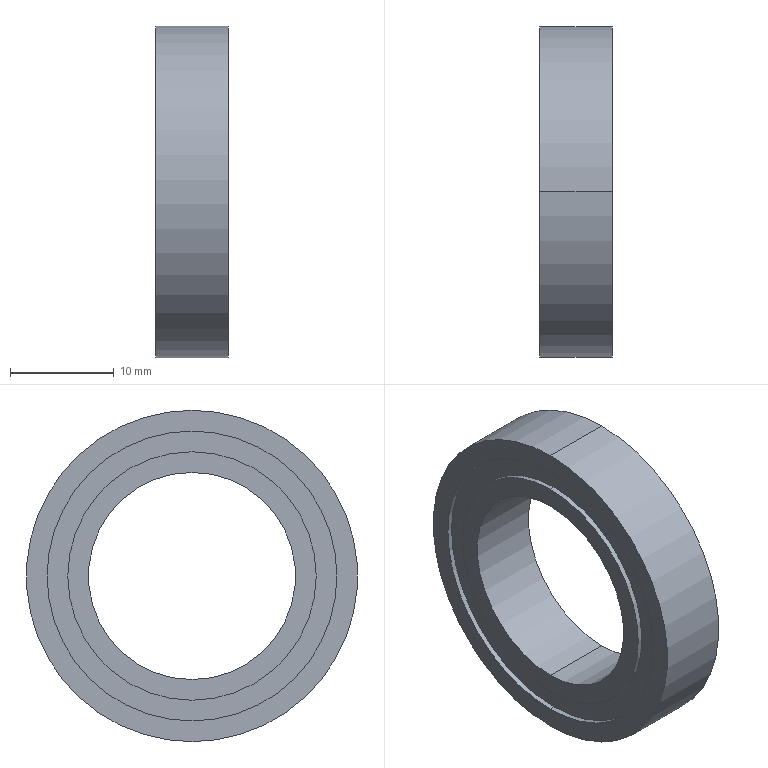Part | SolidWorks | features Revolution 1 | 1 solid | 18 faces | box 7 x 32 x 32 mm | volume 3267 mm3 | cylinder 12 | plane 6 | commonest cylinder face diameters 24 x4 28 x4 20 x2 32 x2
STEP:
#1=CARTESIAN_POINT('',(21.644,0.,-10.));
#2=VERTEX_POINT('',#1);
#3=CARTESIAN_POINT('',(21.644,0.,10.));
#4=VERTEX_POINT('',#3);
#5=CARTESIAN_POINT('',(21.644,0.,0.));
#6=DIRECTION('',(-1.,0.,0.));
#7=DIRECTION('',(0.,0.,1.));
#8=AXIS2_PLACEMENT_3D('',#5,#6,#7);
#9=CIRCLE('',#8,10.);
#10=EDGE_CURVE('',#2,#4,#9,.T.);
#11=ORIENTED_EDGE('',*,*,#10,.F.);
#12=CARTESIAN_POINT('',(14.644,0.,-10.));
#13=VERTEX_POINT('',#12);
#14=CARTESIAN_POINT('',(0.,0.,-10.));
#15=DIRECTION('',(-1.,0.,0.));
#16=VECTOR('',#15,1000.);
#17=LINE('',#14,#16);
#18=EDGE_CURVE('',#2,#13,#17,.T.);
#19=ORIENTED_EDGE('',*,*,#18,.T.);
#20=CARTESIAN_POINT('',(14.644,0.,10.));
#21=VERTEX_POINT('',#20);
#22=CARTESIAN_POINT('',(14.644,0.,0.));
#23=DIRECTION('',(-1.,0.,0.));
#24=DIRECTION('',(0.,0.,1.));
#25=AXIS2_PLACEMENT_3D('',#22,#23,#24);
#26=CIRCLE('',#25,10.);
#27=EDGE_CURVE('',#13,#21,#26,.T.);
#28=ORIENTED_EDGE('',*,*,#27,.T.);
#29=CARTESIAN_POINT('',(0.,0.,10.));
#30=DIRECTION('',(-1.,0.,0.));
#31=VECTOR('',#30,1000.);
#32=LINE('',#29,#31);
#33=EDGE_CURVE('',#4,#21,#32,.T.);
#34=ORIENTED_EDGE('',*,*,#33,.F.);
#35=EDGE_LOOP('',(#11,#19,#28,#34));
#36=FACE_OUTER_BOUND('',#35,.T.);
#37=CARTESIAN_POINT('',(0.,0.,0.));
#38=DIRECTION('',(-1.,0.,0.));
#39=DIRECTION('',(0.,0.,1.));
#40=AXIS2_PLACEMENT_3D('',#37,#38,#39);
#41=CYLINDRICAL_SURFACE('',#40,10.);
#42=ADVANCED_FACE('',(#36),#41,.F.);
#43=CARTESIAN_POINT('',(21.644,0.,12.));
#44=VERTEX_POINT('',#43);
#45=CARTESIAN_POINT('',(21.644,0.,-12.));
#46=VERTEX_POINT('',#45);
#47=CARTESIAN_POINT('',(21.644,0.,0.));
#48=DIRECTION('',(-1.,0.,0.));
#49=DIRECTION('',(0.,0.,1.));
#50=AXIS2_PLACEMENT_3D('',#47,#48,#49);
#51=CIRCLE('',#50,12.);
#52=EDGE_CURVE('',#44,#46,#51,.T.);
#53=ORIENTED_EDGE('',*,*,#52,.T.);
#54=CARTESIAN_POINT('',(21.144,0.,-12.));
#55=VERTEX_POINT('',#54);
#56=CARTESIAN_POINT('',(0.,0.,-12.));
#57=DIRECTION('',(-1.,0.,0.));
#58=VECTOR('',#57,1000.);
#59=LINE('',#56,#58);
#60=EDGE_CURVE('',#46,#55,#59,.T.);
#61=ORIENTED_EDGE('',*,*,#60,.T.);
#62=CARTESIAN_POINT('',(21.144,0.,12.));
#63=VERTEX_POINT('',#62);
#64=CARTESIAN_POINT('',(21.144,0.,0.));
#65=DIRECTION('',(-1.,0.,0.));
#66=DIRECTION('',(0.,0.,1.));
#67=AXIS2_PLACEMENT_3D('',#64,#65,#66);
#68=CIRCLE('',#67,12.);
#69=EDGE_CURVE('',#63,#55,#68,.T.);
#70=ORIENTED_EDGE('',*,*,#69,.F.);
#71=CARTESIAN_POINT('',(0.,0.,12.));
#72=DIRECTION('',(-1.,0.,0.));
#73=VECTOR('',#72,1000.);
#74=LINE('',#71,#73);
#75=EDGE_CURVE('',#44,#63,#74,.T.);
#76=ORIENTED_EDGE('',*,*,#75,.F.);
#77=EDGE_LOOP('',(#53,#61,#70,#76));
#78=FACE_OUTER_BOUND('',#77,.T.);
#79=CARTESIAN_POINT('',(0.,0.,0.));
#80=DIRECTION('',(-1.,0.,0.));
#81=DIRECTION('',(0.,0.,1.));
#82=AXIS2_PLACEMENT_3D('',#79,#80,#81);
#83=CYLINDRICAL_SURFACE('',#82,12.);
#84=ADVANCED_FACE('',(#78),#83,.T.);
#85=CARTESIAN_POINT('',(21.644,0.,-14.));
#86=VERTEX_POINT('',#85);
#87=CARTESIAN_POINT('',(21.644,0.,14.));
#88=VERTEX_POINT('',#87);
#89=CARTESIAN_POINT('',(21.644,0.,0.));
#90=DIRECTION('',(-1.,0.,0.));
#91=DIRECTION('',(0.,0.,1.));
#92=AXIS2_PLACEMENT_3D('',#89,#90,#91);
#93=CIRCLE('',#92,14.);
#94=EDGE_CURVE('',#86,#88,#93,.T.);
#95=ORIENTED_EDGE('',*,*,#94,.F.);
#96=CARTESIAN_POINT('',(21.144,0.,-14.));
#97=VERTEX_POINT('',#96);
#98=CARTESIAN_POINT('',(0.,0.,-14.));
#99=DIRECTION('',(-1.,0.,0.));
#100=VECTOR('',#99,1000.);
#101=LINE('',#98,#100);
#102=EDGE_CURVE('',#86,#97,#101,.T.);
#103=ORIENTED_EDGE('',*,*,#102,.T.);
#104=CARTESIAN_POINT('',(21.144,0.,14.));
#105=VERTEX_POINT('',#104);
#106=CARTESIAN_POINT('',(21.144,0.,0.));
#107=DIRECTION('',(-1.,0.,0.));
#108=DIRECTION('',(0.,0.,1.));
#109=AXIS2_PLACEMENT_3D('',#106,#107,#108);
#110=CIRCLE('',#109,14.);
#111=EDGE_CURVE('',#97,#105,#110,.T.);
#112=ORIENTED_EDGE('',*,*,#111,.T.);
#113=CARTESIAN_POINT('',(0.,0.,14.));
#114=DIRECTION('',(-1.,0.,0.));
#115=VECTOR('',#114,1000.);
#116=LINE('',#113,#115);
#117=EDGE_CURVE('',#88,#105,#116,.T.);
#118=ORIENTED_EDGE('',*,*,#117,.F.);
#119=EDGE_LOOP('',(#95,#103,#112,#118));
#120=FACE_OUTER_BOUND('',#119,.T.);
#121=CARTESIAN_POINT('',(0.,0.,0.));
#122=DIRECTION('',(-1.,0.,0.));
#123=DIRECTION('',(0.,0.,1.));
#124=AXIS2_PLACEMENT_3D('',#121,#122,#123);
#125=CYLINDRICAL_SURFACE('',#124,14.);
#126=ADVANCED_FACE('',(#120),#125,.F.);
#127=CARTESIAN_POINT('',(21.644,0.,16.));
#128=VERTEX_POINT('',#127);
#129=CARTESIAN_POINT('',(21.644,0.,-16.));
#130=VERTEX_POINT('',#129);
#131=CARTESIAN_POINT('',(21.644,0.,0.));
#132=DIRECTION('',(-1.,0.,0.));
#133=DIRECTION('',(0.,0.,1.));
#134=AXIS2_PLACEMENT_3D('',#131,#132,#133);
#135=CIRCLE('',#134,16.);
#136=EDGE_CURVE('',#128,#130,#135,.T.);
#137=ORIENTED_EDGE('',*,*,#136,.T.);
#138=CARTESIAN_POINT('',(14.644,0.,-16.));
#139=VERTEX_POINT('',#138);
#140=CARTESIAN_POINT('',(0.,0.,-16.));
#141=DIRECTION('',(-1.,0.,0.));
#142=VECTOR('',#141,1000.);
#143=LINE('',#140,#142);
#144=EDGE_CURVE('',#130,#139,#143,.T.);
#145=ORIENTED_EDGE('',*,*,#144,.T.);
#146=CARTESIAN_POINT('',(14.644,0.,16.));
#147=VERTEX_POINT('',#146);
#148=CARTESIAN_POINT('',(14.644,0.,0.));
#149=DIRECTION('',(-1.,0.,0.));
#150=DIRECTION('',(0.,0.,1.));
#151=AXIS2_PLACEMENT_3D('',#148,#149,#150);
#152=CIRCLE('',#151,16.);
#153=EDGE_CURVE('',#147,#139,#152,.T.);
#154=ORIENTED_EDGE('',*,*,#153,.F.);
#155=CARTESIAN_POINT('',(0.,0.,16.));
#156=DIRECTION('',(-1.,0.,0.));
#157=VECTOR('',#156,1000.);
#158=LINE('',#155,#157);
#159=EDGE_CURVE('',#128,#147,#158,.T.);
#160=ORIENTED_EDGE('',*,*,#159,.F.);
#161=EDGE_LOOP('',(#137,#145,#154,#160));
#162=FACE_OUTER_BOUND('',#161,.T.);
#163=CARTESIAN_POINT('',(0.,0.,0.));
#164=DIRECTION('',(-1.,0.,0.));
#165=DIRECTION('',(0.,0.,1.));
#166=AXIS2_PLACEMENT_3D('',#163,#164,#165);
#167=CYLINDRICAL_SURFACE('',#166,16.);
#168=ADVANCED_FACE('',(#162),#167,.T.);
#169=CARTESIAN_POINT('',(15.144,0.,-14.));
#170=VERTEX_POINT('',#169);
#171=CARTESIAN_POINT('',(15.144,0.,14.));
#172=VERTEX_POINT('',#171);
#173=CARTESIAN_POINT('',(15.144,0.,0.));
#174=DIRECTION('',(-1.,0.,0.));
#175=DIRECTION('',(0.,0.,1.));
#176=AXIS2_PLACEMENT_3D('',#173,#174,#175);
#177=CIRCLE('',#176,14.);
#178=EDGE_CURVE('',#170,#172,#177,.T.);
#179=ORIENTED_EDGE('',*,*,#178,.F.);
#180=CARTESIAN_POINT('',(14.644,0.,-14.));
#181=VERTEX_POINT('',#180);
#182=CARTESIAN_POINT('',(0.,0.,-14.));
#183=DIRECTION('',(-1.,0.,0.));
#184=VECTOR('',#183,1000.);
#185=LINE('',#182,#184);
#186=EDGE_CURVE('',#170,#181,#185,.T.);
#187=ORIENTED_EDGE('',*,*,#186,.T.);
#188=CARTESIAN_POINT('',(14.644,0.,14.));
#189=VERTEX_POINT('',#188);
#190=CARTESIAN_POINT('',(14.644,0.,0.));
#191=DIRECTION('',(-1.,0.,0.));
#192=DIRECTION('',(0.,0.,1.));
#193=AXIS2_PLACEMENT_3D('',#190,#191,#192);
#194=CIRCLE('',#193,14.);
#195=EDGE_CURVE('',#181,#189,#194,.T.);
#196=ORIENTED_EDGE('',*,*,#195,.T.);
#197=CARTESIAN_POINT('',(0.,0.,14.));
#198=DIRECTION('',(-1.,0.,0.));
#199=VECTOR('',#198,1000.);
#200=LINE('',#197,#199);
#201=EDGE_CURVE('',#172,#189,#200,.T.);
#202=ORIENTED_EDGE('',*,*,#201,.F.);
#203=EDGE_LOOP('',(#179,#187,#196,#202));
#204=FACE_OUTER_BOUND('',#203,.T.);
#205=CARTESIAN_POINT('',(0.,0.,0.));
#206=DIRECTION('',(-1.,0.,0.));
#207=DIRECTION('',(0.,0.,1.));
#208=AXIS2_PLACEMENT_3D('',#205,#206,#207);
#209=CYLINDRICAL_SURFACE('',#208,14.);
#210=ADVANCED_FACE('',(#204),#209,.F.);
#211=CARTESIAN_POINT('',(15.144,0.,12.));
#212=VERTEX_POINT('',#211);
#213=CARTESIAN_POINT('',(15.144,0.,-12.));
#214=VERTEX_POINT('',#213);
#215=CARTESIAN_POINT('',(15.144,0.,0.));
#216=DIRECTION('',(-1.,0.,0.));
#217=DIRECTION('',(0.,0.,1.));
#218=AXIS2_PLACEMENT_3D('',#215,#216,#217);
#219=CIRCLE('',#218,12.);
#220=EDGE_CURVE('',#212,#214,#219,.T.);
#221=ORIENTED_EDGE('',*,*,#220,.T.);
#222=CARTESIAN_POINT('',(14.644,0.,-12.));
#223=VERTEX_POINT('',#222);
#224=CARTESIAN_POINT('',(0.,0.,-12.));
#225=DIRECTION('',(-1.,0.,0.));
#226=VECTOR('',#225,1000.);
#227=LINE('',#224,#226);
#228=EDGE_CURVE('',#214,#223,#227,.T.);
#229=ORIENTED_EDGE('',*,*,#228,.T.);
#230=CARTESIAN_POINT('',(14.644,0.,12.));
#231=VERTEX_POINT('',#230);
#232=CARTESIAN_POINT('',(14.644,0.,0.));
#233=DIRECTION('',(-1.,0.,0.));
#234=DIRECTION('',(0.,0.,1.));
#235=AXIS2_PLACEMENT_3D('',#232,#233,#234);
#236=CIRCLE('',#235,12.);
#237=EDGE_CURVE('',#231,#223,#236,.T.);
#238=ORIENTED_EDGE('',*,*,#237,.F.);
#239=CARTESIAN_POINT('',(0.,0.,12.));
#240=DIRECTION('',(-1.,0.,0.));
#241=VECTOR('',#240,1000.);
#242=LINE('',#239,#241);
#243=EDGE_CURVE('',#212,#231,#242,.T.);
#244=ORIENTED_EDGE('',*,*,#243,.F.);
#245=EDGE_LOOP('',(#221,#229,#238,#244));
#246=FACE_OUTER_BOUND('',#245,.T.);
#247=CARTESIAN_POINT('',(0.,0.,0.));
#248=DIRECTION('',(-1.,0.,0.));
#249=DIRECTION('',(0.,0.,1.));
#250=AXIS2_PLACEMENT_3D('',#247,#248,#249);
#251=CYLINDRICAL_SURFACE('',#250,12.);
#252=ADVANCED_FACE('',(#246),#251,.T.);
#253=CARTESIAN_POINT('',(14.644,0.,0.));
#254=DIRECTION('',(-1.,0.,0.));
#255=DIRECTION('',(0.,0.,1.));
#256=AXIS2_PLACEMENT_3D('',#253,#254,#255);
#257=CIRCLE('',#256,10.);
#258=EDGE_CURVE('',#21,#13,#257,.T.);
#259=ORIENTED_EDGE('',*,*,#258,.F.);
#260=ORIENTED_EDGE('',*,*,#27,.F.);
#261=EDGE_LOOP('',(#259,#260));
#262=FACE_BOUND('',#261,.T.);
#263=ORIENTED_EDGE('',*,*,#237,.T.);
#264=CARTESIAN_POINT('',(14.644,0.,0.));
#265=DIRECTION('',(-1.,0.,0.));
#266=DIRECTION('',(0.,0.,1.));
#267=AXIS2_PLACEMENT_3D('',#264,#265,#266);
#268=CIRCLE('',#267,12.);
#269=EDGE_CURVE('',#223,#231,#268,.T.);
#270=ORIENTED_EDGE('',*,*,#269,.T.);
#271=EDGE_LOOP('',(#263,#270));
#272=FACE_OUTER_BOUND('',#271,.T.);
#273=CARTESIAN_POINT('',(14.644,10.,0.));
#274=DIRECTION('',(1.,0.,0.));
#275=DIRECTION('',(0.,0.,-1.));
#276=AXIS2_PLACEMENT_3D('',#273,#274,#275);
#277=PLANE('',#276);
#278=ADVANCED_FACE('',(#262,#272),#277,.F.);
#279=ORIENTED_EDGE('',*,*,#228,.F.);
#280=CARTESIAN_POINT('',(15.144,0.,0.));
#281=DIRECTION('',(-1.,0.,0.));
#282=DIRECTION('',(0.,0.,1.));
#283=AXIS2_PLACEMENT_3D('',#280,#281,#282);
#284=CIRCLE('',#283,12.);
#285=EDGE_CURVE('',#214,#212,#284,.T.);
#286=ORIENTED_EDGE('',*,*,#285,.T.);
#287=ORIENTED_EDGE('',*,*,#243,.T.);
#288=ORIENTED_EDGE('',*,*,#269,.F.);
#289=EDGE_LOOP('',(#279,#286,#287,#288));
#290=FACE_OUTER_BOUND('',#289,.T.);
#291=CARTESIAN_POINT('',(0.,0.,0.));
#292=DIRECTION('',(-1.,0.,0.));
#293=DIRECTION('',(0.,0.,1.));
#294=AXIS2_PLACEMENT_3D('',#291,#292,#293);
#295=CYLINDRICAL_SURFACE('',#294,12.);
#296=ADVANCED_FACE('',(#290),#295,.T.);
#297=ORIENTED_EDGE('',*,*,#220,.F.);
#298=ORIENTED_EDGE('',*,*,#285,.F.);
#299=EDGE_LOOP('',(#297,#298));
#300=FACE_BOUND('',#299,.T.);
#301=CARTESIAN_POINT('',(15.144,0.,0.));
#302=DIRECTION('',(-1.,0.,0.));
#303=DIRECTION('',(0.,0.,1.));
#304=AXIS2_PLACEMENT_3D('',#301,#302,#303);
#305=CIRCLE('',#304,14.);
#306=EDGE_CURVE('',#172,#170,#305,.T.);
#307=ORIENTED_EDGE('',*,*,#306,.T.);
#308=ORIENTED_EDGE('',*,*,#178,.T.);
#309=EDGE_LOOP('',(#307,#308));
#310=FACE_OUTER_BOUND('',#309,.T.);
#311=CARTESIAN_POINT('',(15.144,12.,0.));
#312=DIRECTION('',(1.,0.,0.));
#313=DIRECTION('',(0.,0.,-1.));
#314=AXIS2_PLACEMENT_3D('',#311,#312,#313);
#315=PLANE('',#314);
#316=ADVANCED_FACE('',(#300,#310),#315,.F.);
#317=ORIENTED_EDGE('',*,*,#186,.F.);
#318=ORIENTED_EDGE('',*,*,#306,.F.);
#319=ORIENTED_EDGE('',*,*,#201,.T.);
#320=CARTESIAN_POINT('',(14.644,0.,0.));
#321=DIRECTION('',(-1.,0.,0.));
#322=DIRECTION('',(0.,0.,1.));
#323=AXIS2_PLACEMENT_3D('',#320,#321,#322);
#324=CIRCLE('',#323,14.);
#325=EDGE_CURVE('',#189,#181,#324,.T.);
#326=ORIENTED_EDGE('',*,*,#325,.T.);
#327=EDGE_LOOP('',(#317,#318,#319,#326));
#328=FACE_OUTER_BOUND('',#327,.T.);
#329=CARTESIAN_POINT('',(0.,0.,0.));
#330=DIRECTION('',(-1.,0.,0.));
#331=DIRECTION('',(0.,0.,1.));
#332=AXIS2_PLACEMENT_3D('',#329,#330,#331);
#333=CYLINDRICAL_SURFACE('',#332,14.);
#334=ADVANCED_FACE('',(#328),#333,.F.);
#335=ORIENTED_EDGE('',*,*,#325,.F.);
#336=ORIENTED_EDGE('',*,*,#195,.F.);
#337=EDGE_LOOP('',(#335,#336));
#338=FACE_BOUND('',#337,.T.);
#339=ORIENTED_EDGE('',*,*,#153,.T.);
#340=CARTESIAN_POINT('',(14.644,0.,0.));
#341=DIRECTION('',(-1.,0.,0.));
#342=DIRECTION('',(0.,0.,1.));
#343=AXIS2_PLACEMENT_3D('',#340,#341,#342);
#344=CIRCLE('',#343,16.);
#345=EDGE_CURVE('',#139,#147,#344,.T.);
#346=ORIENTED_EDGE('',*,*,#345,.T.);
#347=EDGE_LOOP('',(#339,#346));
#348=FACE_OUTER_BOUND('',#347,.T.);
#349=CARTESIAN_POINT('',(14.644,14.,0.));
#350=DIRECTION('',(1.,0.,0.));
#351=DIRECTION('',(0.,0.,-1.));
#352=AXIS2_PLACEMENT_3D('',#349,#350,#351);
#353=PLANE('',#352);
#354=ADVANCED_FACE('',(#338,#348),#353,.F.);
#355=ORIENTED_EDGE('',*,*,#144,.F.);
#356=CARTESIAN_POINT('',(21.644,0.,0.));
#357=DIRECTION('',(-1.,0.,0.));
#358=DIRECTION('',(0.,0.,1.));
#359=AXIS2_PLACEMENT_3D('',#356,#357,#358);
#360=CIRCLE('',#359,16.);
#361=EDGE_CURVE('',#130,#128,#360,.T.);
#362=ORIENTED_EDGE('',*,*,#361,.T.);
#363=ORIENTED_EDGE('',*,*,#159,.T.);
#364=ORIENTED_EDGE('',*,*,#345,.F.);
#365=EDGE_LOOP('',(#355,#362,#363,#364));
#366=FACE_OUTER_BOUND('',#365,.T.);
#367=CARTESIAN_POINT('',(0.,0.,0.));
#368=DIRECTION('',(-1.,0.,0.));
#369=DIRECTION('',(0.,0.,1.));
#370=AXIS2_PLACEMENT_3D('',#367,#368,#369);
#371=CYLINDRICAL_SURFACE('',#370,16.);
#372=ADVANCED_FACE('',(#366),#371,.T.);
#373=ORIENTED_EDGE('',*,*,#136,.F.);
#374=ORIENTED_EDGE('',*,*,#361,.F.);
#375=EDGE_LOOP('',(#373,#374));
#376=FACE_OUTER_BOUND('',#375,.T.);
#377=CARTESIAN_POINT('',(21.644,0.,0.));
#378=DIRECTION('',(-1.,0.,0.));
#379=DIRECTION('',(0.,0.,1.));
#380=AXIS2_PLACEMENT_3D('',#377,#378,#379);
#381=CIRCLE('',#380,14.);
#382=EDGE_CURVE('',#88,#86,#381,.T.);
#383=ORIENTED_EDGE('',*,*,#382,.T.);
#384=ORIENTED_EDGE('',*,*,#94,.T.);
#385=EDGE_LOOP('',(#383,#384));
#386=FACE_BOUND('',#385,.T.);
#387=CARTESIAN_POINT('',(21.644,14.,0.));
#388=DIRECTION('',(-1.,0.,0.));
#389=DIRECTION('',(0.,0.,1.));
#390=AXIS2_PLACEMENT_3D('',#387,#388,#389);
#391=PLANE('',#390);
#392=ADVANCED_FACE('',(#376,#386),#391,.F.);
#393=ORIENTED_EDGE('',*,*,#102,.F.);
#394=ORIENTED_EDGE('',*,*,#382,.F.);
#395=ORIENTED_EDGE('',*,*,#117,.T.);
#396=CARTESIAN_POINT('',(21.144,0.,0.));
#397=DIRECTION('',(-1.,0.,0.));
#398=DIRECTION('',(0.,0.,1.));
#399=AXIS2_PLACEMENT_3D('',#396,#397,#398);
#400=CIRCLE('',#399,14.);
#401=EDGE_CURVE('',#105,#97,#400,.T.);
#402=ORIENTED_EDGE('',*,*,#401,.T.);
#403=EDGE_LOOP('',(#393,#394,#395,#402));
#404=FACE_OUTER_BOUND('',#403,.T.);
#405=CARTESIAN_POINT('',(0.,0.,0.));
#406=DIRECTION('',(-1.,0.,0.));
#407=DIRECTION('',(0.,0.,1.));
#408=AXIS2_PLACEMENT_3D('',#405,#406,#407);
#409=CYLINDRICAL_SURFACE('',#408,14.);
#410=ADVANCED_FACE('',(#404),#409,.F.);
#411=ORIENTED_EDGE('',*,*,#401,.F.);
#412=ORIENTED_EDGE('',*,*,#111,.F.);
#413=EDGE_LOOP('',(#411,#412));
#414=FACE_OUTER_BOUND('',#413,.T.);
#415=ORIENTED_EDGE('',*,*,#69,.T.);
#416=CARTESIAN_POINT('',(21.144,0.,0.));
#417=DIRECTION('',(-1.,0.,0.));
#418=DIRECTION('',(0.,0.,1.));
#419=AXIS2_PLACEMENT_3D('',#416,#417,#418);
#420=CIRCLE('',#419,12.);
#421=EDGE_CURVE('',#55,#63,#420,.T.);
#422=ORIENTED_EDGE('',*,*,#421,.T.);
#423=EDGE_LOOP('',(#415,#422));
#424=FACE_BOUND('',#423,.T.);
#425=CARTESIAN_POINT('',(21.144,12.,0.));
#426=DIRECTION('',(-1.,0.,0.));
#427=DIRECTION('',(0.,0.,1.));
#428=AXIS2_PLACEMENT_3D('',#425,#426,#427);
#429=PLANE('',#428);
#430=ADVANCED_FACE('',(#414,#424),#429,.F.);
#431=ORIENTED_EDGE('',*,*,#60,.F.);
#432=CARTESIAN_POINT('',(21.644,0.,0.));
#433=DIRECTION('',(-1.,0.,0.));
#434=DIRECTION('',(0.,0.,1.));
#435=AXIS2_PLACEMENT_3D('',#432,#433,#434);
#436=CIRCLE('',#435,12.);
#437=EDGE_CURVE('',#46,#44,#436,.T.);
#438=ORIENTED_EDGE('',*,*,#437,.T.);
#439=ORIENTED_EDGE('',*,*,#75,.T.);
#440=ORIENTED_EDGE('',*,*,#421,.F.);
#441=EDGE_LOOP('',(#431,#438,#439,#440));
#442=FACE_OUTER_BOUND('',#441,.T.);
#443=CARTESIAN_POINT('',(0.,0.,0.));
#444=DIRECTION('',(-1.,0.,0.));
#445=DIRECTION('',(0.,0.,1.));
#446=AXIS2_PLACEMENT_3D('',#443,#444,#445);
#447=CYLINDRICAL_SURFACE('',#446,12.);
#448=ADVANCED_FACE('',(#442),#447,.T.);
#449=ORIENTED_EDGE('',*,*,#52,.F.);
#450=ORIENTED_EDGE('',*,*,#437,.F.);
#451=EDGE_LOOP('',(#449,#450));
#452=FACE_OUTER_BOUND('',#451,.T.);
#453=CARTESIAN_POINT('',(21.644,0.,0.));
#454=DIRECTION('',(-1.,0.,0.));
#455=DIRECTION('',(0.,0.,1.));
#456=AXIS2_PLACEMENT_3D('',#453,#454,#455);
#457=CIRCLE('',#456,10.);
#458=EDGE_CURVE('',#4,#2,#457,.T.);
#459=ORIENTED_EDGE('',*,*,#458,.T.);
#460=ORIENTED_EDGE('',*,*,#10,.T.);
#461=EDGE_LOOP('',(#459,#460));
#462=FACE_BOUND('',#461,.T.);
#463=CARTESIAN_POINT('',(21.644,10.,0.));
#464=DIRECTION('',(-1.,0.,0.));
#465=DIRECTION('',(0.,0.,1.));
#466=AXIS2_PLACEMENT_3D('',#463,#464,#465);
#467=PLANE('',#466);
#468=ADVANCED_FACE('',(#452,#462),#467,.F.);
#469=ORIENTED_EDGE('',*,*,#18,.F.);
#470=ORIENTED_EDGE('',*,*,#458,.F.);
#471=ORIENTED_EDGE('',*,*,#33,.T.);
#472=ORIENTED_EDGE('',*,*,#258,.T.);
#473=EDGE_LOOP('',(#469,#470,#471,#472));
#474=FACE_OUTER_BOUND('',#473,.T.);
#475=CARTESIAN_POINT('',(0.,0.,0.));
#476=DIRECTION('',(-1.,0.,0.));
#477=DIRECTION('',(0.,0.,1.));
#478=AXIS2_PLACEMENT_3D('',#475,#476,#477);
#479=CYLINDRICAL_SURFACE('',#478,10.);
#480=ADVANCED_FACE('',(#474),#479,.F.);
#481=CLOSED_SHELL('',(#42,#84,#126,#168,#210,#252,#278,#296,#316,#334,#354,#372,#392,#410,#430,#448,#468,#480));
#482=MANIFOLD_SOLID_BREP('',#481);
#483=CARTESIAN_POINT('',(0.,0.,0.));
#484=DIRECTION('',(0.,0.,1.));
#485=DIRECTION('',(1.,0.,0.));
#486=AXIS2_PLACEMENT_3D('',#483,#484,#485);
#487=(LENGTH_UNIT()NAMED_UNIT(*)SI_UNIT(.MILLI.,.METRE.));
#488=UNCERTAINTY_MEASURE_WITH_UNIT(LENGTH_MEASURE(0.00001),#487,'','');
#489=(NAMED_UNIT(*)PLANE_ANGLE_UNIT()SI_UNIT($,.RADIAN.));
#490=(NAMED_UNIT(*)SI_UNIT($,.STERADIAN.)SOLID_ANGLE_UNIT());
#491=(GEOMETRIC_REPRESENTATION_CONTEXT(3)GLOBAL_UNCERTAINTY_ASSIGNED_CONTEXT((#488))GLOBAL_UNIT_ASSIGNED_CONTEXT((#487,#489,#490))REPRESENTATION_CONTEXT('',''));
#492=ADVANCED_BREP_SHAPE_REPRESENTATION('',(#482,#486),#491);